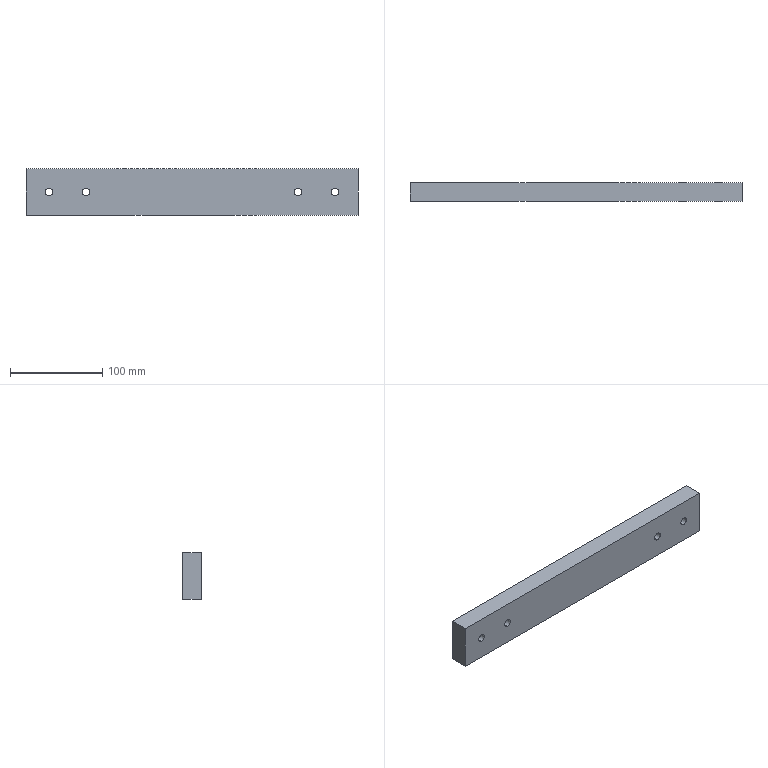Part | SolidWorks | features Extrusion 1, HoleWzd 1 | 1 solid | 14 faces | box 360 x 20 x 50 mm | volume 355460 mm3 | cylinder 8 | plane 6 | commonest cylinder face diameters 8.5 x8
STEP:
#1=CARTESIAN_POINT('',(335.,67.,-20.75));
#2=VERTEX_POINT('',#1);
#3=CARTESIAN_POINT('',(335.,67.,-29.25));
#4=VERTEX_POINT('',#3);
#5=CARTESIAN_POINT('',(335.,67.,-25.));
#6=DIRECTION('',(0.,-1.,0.));
#7=DIRECTION('',(0.,0.,-1.));
#8=AXIS2_PLACEMENT_3D('',#5,#6,#7);
#9=CIRCLE('',#8,4.25);
#10=EDGE_CURVE('',#2,#4,#9,.T.);
#11=ORIENTED_EDGE('',*,*,#10,.F.);
#12=CARTESIAN_POINT('',(335.,47.,-20.75));
#13=VERTEX_POINT('',#12);
#14=CARTESIAN_POINT('',(335.,47.,-20.75));
#15=DIRECTION('',(0.,-1.,0.));
#16=VECTOR('',#15,1000.);
#17=LINE('',#14,#16);
#18=EDGE_CURVE('',#2,#13,#17,.T.);
#19=ORIENTED_EDGE('',*,*,#18,.T.);
#20=CARTESIAN_POINT('',(335.,47.,-29.25));
#21=VERTEX_POINT('',#20);
#22=CARTESIAN_POINT('',(335.,47.,-25.));
#23=DIRECTION('',(0.,-1.,0.));
#24=DIRECTION('',(0.,0.,-1.));
#25=AXIS2_PLACEMENT_3D('',#22,#23,#24);
#26=CIRCLE('',#25,4.25);
#27=EDGE_CURVE('',#13,#21,#26,.T.);
#28=ORIENTED_EDGE('',*,*,#27,.T.);
#29=CARTESIAN_POINT('',(335.,47.,-29.25));
#30=DIRECTION('',(0.,-1.,0.));
#31=VECTOR('',#30,1000.);
#32=LINE('',#29,#31);
#33=EDGE_CURVE('',#4,#21,#32,.T.);
#34=ORIENTED_EDGE('',*,*,#33,.F.);
#35=EDGE_LOOP('',(#11,#19,#28,#34));
#36=FACE_OUTER_BOUND('',#35,.T.);
#37=CARTESIAN_POINT('',(335.,47.,-25.));
#38=DIRECTION('',(0.,-1.,0.));
#39=DIRECTION('',(0.,0.,-1.));
#40=AXIS2_PLACEMENT_3D('',#37,#38,#39);
#41=CYLINDRICAL_SURFACE('',#40,4.25);
#42=ADVANCED_FACE('',(#36),#41,.F.);
#43=CARTESIAN_POINT('',(295.,67.,-20.75));
#44=VERTEX_POINT('',#43);
#45=CARTESIAN_POINT('',(295.,67.,-29.25));
#46=VERTEX_POINT('',#45);
#47=CARTESIAN_POINT('',(295.,67.,-25.));
#48=DIRECTION('',(0.,-1.,0.));
#49=DIRECTION('',(0.,0.,-1.));
#50=AXIS2_PLACEMENT_3D('',#47,#48,#49);
#51=CIRCLE('',#50,4.25);
#52=EDGE_CURVE('',#44,#46,#51,.T.);
#53=ORIENTED_EDGE('',*,*,#52,.F.);
#54=CARTESIAN_POINT('',(295.,47.,-20.75));
#55=VERTEX_POINT('',#54);
#56=CARTESIAN_POINT('',(295.,47.,-20.75));
#57=DIRECTION('',(0.,-1.,0.));
#58=VECTOR('',#57,1000.);
#59=LINE('',#56,#58);
#60=EDGE_CURVE('',#44,#55,#59,.T.);
#61=ORIENTED_EDGE('',*,*,#60,.T.);
#62=CARTESIAN_POINT('',(295.,47.,-29.25));
#63=VERTEX_POINT('',#62);
#64=CARTESIAN_POINT('',(295.,47.,-25.));
#65=DIRECTION('',(0.,-1.,0.));
#66=DIRECTION('',(0.,0.,-1.));
#67=AXIS2_PLACEMENT_3D('',#64,#65,#66);
#68=CIRCLE('',#67,4.25);
#69=EDGE_CURVE('',#55,#63,#68,.T.);
#70=ORIENTED_EDGE('',*,*,#69,.T.);
#71=CARTESIAN_POINT('',(295.,47.,-29.25));
#72=DIRECTION('',(0.,-1.,0.));
#73=VECTOR('',#72,1000.);
#74=LINE('',#71,#73);
#75=EDGE_CURVE('',#46,#63,#74,.T.);
#76=ORIENTED_EDGE('',*,*,#75,.F.);
#77=EDGE_LOOP('',(#53,#61,#70,#76));
#78=FACE_OUTER_BOUND('',#77,.T.);
#79=CARTESIAN_POINT('',(295.,47.,-25.));
#80=DIRECTION('',(0.,-1.,0.));
#81=DIRECTION('',(0.,0.,-1.));
#82=AXIS2_PLACEMENT_3D('',#79,#80,#81);
#83=CYLINDRICAL_SURFACE('',#82,4.25);
#84=ADVANCED_FACE('',(#78),#83,.F.);
#85=CARTESIAN_POINT('',(65.,67.,-20.75));
#86=VERTEX_POINT('',#85);
#87=CARTESIAN_POINT('',(65.,67.,-29.25));
#88=VERTEX_POINT('',#87);
#89=CARTESIAN_POINT('',(65.,67.,-25.));
#90=DIRECTION('',(0.,-1.,0.));
#91=DIRECTION('',(0.,0.,-1.));
#92=AXIS2_PLACEMENT_3D('',#89,#90,#91);
#93=CIRCLE('',#92,4.25);
#94=EDGE_CURVE('',#86,#88,#93,.T.);
#95=ORIENTED_EDGE('',*,*,#94,.F.);
#96=CARTESIAN_POINT('',(65.,47.,-20.75));
#97=VERTEX_POINT('',#96);
#98=CARTESIAN_POINT('',(65.,47.,-20.75));
#99=DIRECTION('',(0.,-1.,0.));
#100=VECTOR('',#99,1000.);
#101=LINE('',#98,#100);
#102=EDGE_CURVE('',#86,#97,#101,.T.);
#103=ORIENTED_EDGE('',*,*,#102,.T.);
#104=CARTESIAN_POINT('',(65.,47.,-29.25));
#105=VERTEX_POINT('',#104);
#106=CARTESIAN_POINT('',(65.,47.,-25.));
#107=DIRECTION('',(0.,-1.,0.));
#108=DIRECTION('',(0.,0.,-1.));
#109=AXIS2_PLACEMENT_3D('',#106,#107,#108);
#110=CIRCLE('',#109,4.25);
#111=EDGE_CURVE('',#97,#105,#110,.T.);
#112=ORIENTED_EDGE('',*,*,#111,.T.);
#113=CARTESIAN_POINT('',(65.,47.,-29.25));
#114=DIRECTION('',(0.,-1.,0.));
#115=VECTOR('',#114,1000.);
#116=LINE('',#113,#115);
#117=EDGE_CURVE('',#88,#105,#116,.T.);
#118=ORIENTED_EDGE('',*,*,#117,.F.);
#119=EDGE_LOOP('',(#95,#103,#112,#118));
#120=FACE_OUTER_BOUND('',#119,.T.);
#121=CARTESIAN_POINT('',(65.,47.,-25.));
#122=DIRECTION('',(0.,-1.,0.));
#123=DIRECTION('',(0.,0.,-1.));
#124=AXIS2_PLACEMENT_3D('',#121,#122,#123);
#125=CYLINDRICAL_SURFACE('',#124,4.25);
#126=ADVANCED_FACE('',(#120),#125,.F.);
#127=CARTESIAN_POINT('',(25.,67.,-20.75));
#128=VERTEX_POINT('',#127);
#129=CARTESIAN_POINT('',(25.,67.,-29.25));
#130=VERTEX_POINT('',#129);
#131=CARTESIAN_POINT('',(25.,67.,-25.));
#132=DIRECTION('',(0.,-1.,0.));
#133=DIRECTION('',(0.,0.,-1.));
#134=AXIS2_PLACEMENT_3D('',#131,#132,#133);
#135=CIRCLE('',#134,4.25);
#136=EDGE_CURVE('',#128,#130,#135,.T.);
#137=ORIENTED_EDGE('',*,*,#136,.F.);
#138=CARTESIAN_POINT('',(25.,47.,-20.75));
#139=VERTEX_POINT('',#138);
#140=CARTESIAN_POINT('',(25.,47.,-20.75));
#141=DIRECTION('',(0.,-1.,0.));
#142=VECTOR('',#141,1000.);
#143=LINE('',#140,#142);
#144=EDGE_CURVE('',#128,#139,#143,.T.);
#145=ORIENTED_EDGE('',*,*,#144,.T.);
#146=CARTESIAN_POINT('',(25.,47.,-29.25));
#147=VERTEX_POINT('',#146);
#148=CARTESIAN_POINT('',(25.,47.,-25.));
#149=DIRECTION('',(0.,-1.,0.));
#150=DIRECTION('',(0.,0.,-1.));
#151=AXIS2_PLACEMENT_3D('',#148,#149,#150);
#152=CIRCLE('',#151,4.25);
#153=EDGE_CURVE('',#139,#147,#152,.T.);
#154=ORIENTED_EDGE('',*,*,#153,.T.);
#155=CARTESIAN_POINT('',(25.,47.,-29.25));
#156=DIRECTION('',(0.,-1.,0.));
#157=VECTOR('',#156,1000.);
#158=LINE('',#155,#157);
#159=EDGE_CURVE('',#130,#147,#158,.T.);
#160=ORIENTED_EDGE('',*,*,#159,.F.);
#161=EDGE_LOOP('',(#137,#145,#154,#160));
#162=FACE_OUTER_BOUND('',#161,.T.);
#163=CARTESIAN_POINT('',(25.,47.,-25.));
#164=DIRECTION('',(0.,-1.,0.));
#165=DIRECTION('',(0.,0.,-1.));
#166=AXIS2_PLACEMENT_3D('',#163,#164,#165);
#167=CYLINDRICAL_SURFACE('',#166,4.25);
#168=ADVANCED_FACE('',(#162),#167,.F.);
#169=CARTESIAN_POINT('',(360.,47.,-50.));
#170=VERTEX_POINT('',#169);
#171=CARTESIAN_POINT('',(360.,47.,0.));
#172=VERTEX_POINT('',#171);
#173=CARTESIAN_POINT('',(360.,47.,-50.));
#174=DIRECTION('',(0.,0.,1.));
#175=VECTOR('',#174,1000.);
#176=LINE('',#173,#175);
#177=EDGE_CURVE('',#170,#172,#176,.T.);
#178=ORIENTED_EDGE('',*,*,#177,.F.);
#179=CARTESIAN_POINT('',(360.,67.,-50.));
#180=VERTEX_POINT('',#179);
#181=CARTESIAN_POINT('',(360.,67.,-50.));
#182=DIRECTION('',(0.,-1.,0.));
#183=VECTOR('',#182,1000.);
#184=LINE('',#181,#183);
#185=EDGE_CURVE('',#180,#170,#184,.T.);
#186=ORIENTED_EDGE('',*,*,#185,.F.);
#187=CARTESIAN_POINT('',(360.,67.,0.));
#188=VERTEX_POINT('',#187);
#189=CARTESIAN_POINT('',(360.,67.,-50.));
#190=DIRECTION('',(0.,0.,1.));
#191=VECTOR('',#190,1000.);
#192=LINE('',#189,#191);
#193=EDGE_CURVE('',#180,#188,#192,.T.);
#194=ORIENTED_EDGE('',*,*,#193,.T.);
#195=CARTESIAN_POINT('',(360.,67.,0.));
#196=DIRECTION('',(0.,-1.,0.));
#197=VECTOR('',#196,1000.);
#198=LINE('',#195,#197);
#199=EDGE_CURVE('',#188,#172,#198,.T.);
#200=ORIENTED_EDGE('',*,*,#199,.T.);
#201=EDGE_LOOP('',(#178,#186,#194,#200));
#202=FACE_OUTER_BOUND('',#201,.T.);
#203=CARTESIAN_POINT('',(360.,67.,-50.));
#204=DIRECTION('',(1.,0.,0.));
#205=DIRECTION('',(0.,0.,-1.));
#206=AXIS2_PLACEMENT_3D('',#203,#204,#205);
#207=PLANE('',#206);
#208=ADVANCED_FACE('',(#202),#207,.T.);
#209=CARTESIAN_POINT('',(0.,47.,-50.));
#210=VERTEX_POINT('',#209);
#211=CARTESIAN_POINT('',(0.,47.,-50.));
#212=DIRECTION('',(1.,0.,0.));
#213=VECTOR('',#212,1000.);
#214=LINE('',#211,#213);
#215=EDGE_CURVE('',#210,#170,#214,.T.);
#216=ORIENTED_EDGE('',*,*,#215,.F.);
#217=CARTESIAN_POINT('',(0.,67.,-50.));
#218=VERTEX_POINT('',#217);
#219=CARTESIAN_POINT('',(0.,67.,-50.));
#220=DIRECTION('',(0.,-1.,0.));
#221=VECTOR('',#220,1000.);
#222=LINE('',#219,#221);
#223=EDGE_CURVE('',#218,#210,#222,.T.);
#224=ORIENTED_EDGE('',*,*,#223,.F.);
#225=CARTESIAN_POINT('',(0.,67.,-50.));
#226=DIRECTION('',(1.,0.,0.));
#227=VECTOR('',#226,1000.);
#228=LINE('',#225,#227);
#229=EDGE_CURVE('',#218,#180,#228,.T.);
#230=ORIENTED_EDGE('',*,*,#229,.T.);
#231=ORIENTED_EDGE('',*,*,#185,.T.);
#232=EDGE_LOOP('',(#216,#224,#230,#231));
#233=FACE_OUTER_BOUND('',#232,.T.);
#234=CARTESIAN_POINT('',(0.,67.,-50.));
#235=DIRECTION('',(0.,0.,-1.));
#236=DIRECTION('',(-1.,0.,0.));
#237=AXIS2_PLACEMENT_3D('',#234,#235,#236);
#238=PLANE('',#237);
#239=ADVANCED_FACE('',(#233),#238,.T.);
#240=CARTESIAN_POINT('',(0.,47.,0.));
#241=VERTEX_POINT('',#240);
#242=CARTESIAN_POINT('',(0.,47.,0.));
#243=DIRECTION('',(0.,0.,-1.));
#244=VECTOR('',#243,1000.);
#245=LINE('',#242,#244);
#246=EDGE_CURVE('',#241,#210,#245,.T.);
#247=ORIENTED_EDGE('',*,*,#246,.F.);
#248=CARTESIAN_POINT('',(0.,67.,0.));
#249=VERTEX_POINT('',#248);
#250=CARTESIAN_POINT('',(0.,67.,0.));
#251=DIRECTION('',(0.,-1.,0.));
#252=VECTOR('',#251,1000.);
#253=LINE('',#250,#252);
#254=EDGE_CURVE('',#249,#241,#253,.T.);
#255=ORIENTED_EDGE('',*,*,#254,.F.);
#256=CARTESIAN_POINT('',(0.,67.,0.));
#257=DIRECTION('',(0.,0.,-1.));
#258=VECTOR('',#257,1000.);
#259=LINE('',#256,#258);
#260=EDGE_CURVE('',#249,#218,#259,.T.);
#261=ORIENTED_EDGE('',*,*,#260,.T.);
#262=ORIENTED_EDGE('',*,*,#223,.T.);
#263=EDGE_LOOP('',(#247,#255,#261,#262));
#264=FACE_OUTER_BOUND('',#263,.T.);
#265=CARTESIAN_POINT('',(0.,67.,0.));
#266=DIRECTION('',(-1.,0.,0.));
#267=DIRECTION('',(0.,0.,1.));
#268=AXIS2_PLACEMENT_3D('',#265,#266,#267);
#269=PLANE('',#268);
#270=ADVANCED_FACE('',(#264),#269,.T.);
#271=CARTESIAN_POINT('',(360.,47.,0.));
#272=DIRECTION('',(-1.,0.,0.));
#273=VECTOR('',#272,1000.);
#274=LINE('',#271,#273);
#275=EDGE_CURVE('',#172,#241,#274,.T.);
#276=ORIENTED_EDGE('',*,*,#275,.F.);
#277=ORIENTED_EDGE('',*,*,#199,.F.);
#278=CARTESIAN_POINT('',(360.,67.,0.));
#279=DIRECTION('',(-1.,0.,0.));
#280=VECTOR('',#279,1000.);
#281=LINE('',#278,#280);
#282=EDGE_CURVE('',#188,#249,#281,.T.);
#283=ORIENTED_EDGE('',*,*,#282,.T.);
#284=ORIENTED_EDGE('',*,*,#254,.T.);
#285=EDGE_LOOP('',(#276,#277,#283,#284));
#286=FACE_OUTER_BOUND('',#285,.T.);
#287=CARTESIAN_POINT('',(360.,67.,0.));
#288=DIRECTION('',(0.,0.,1.));
#289=DIRECTION('',(1.,0.,0.));
#290=AXIS2_PLACEMENT_3D('',#287,#288,#289);
#291=PLANE('',#290);
#292=ADVANCED_FACE('',(#286),#291,.T.);
#293=CARTESIAN_POINT('',(335.,67.,-25.));
#294=DIRECTION('',(0.,-1.,0.));
#295=DIRECTION('',(0.,0.,-1.));
#296=AXIS2_PLACEMENT_3D('',#293,#294,#295);
#297=CIRCLE('',#296,4.25);
#298=EDGE_CURVE('',#4,#2,#297,.T.);
#299=ORIENTED_EDGE('',*,*,#298,.T.);
#300=ORIENTED_EDGE('',*,*,#10,.T.);
#301=EDGE_LOOP('',(#299,#300));
#302=FACE_BOUND('',#301,.T.);
#303=CARTESIAN_POINT('',(295.,67.,-25.));
#304=DIRECTION('',(0.,-1.,0.));
#305=DIRECTION('',(0.,0.,-1.));
#306=AXIS2_PLACEMENT_3D('',#303,#304,#305);
#307=CIRCLE('',#306,4.25);
#308=EDGE_CURVE('',#46,#44,#307,.T.);
#309=ORIENTED_EDGE('',*,*,#308,.T.);
#310=ORIENTED_EDGE('',*,*,#52,.T.);
#311=EDGE_LOOP('',(#309,#310));
#312=FACE_BOUND('',#311,.T.);
#313=CARTESIAN_POINT('',(65.,67.,-25.));
#314=DIRECTION('',(0.,-1.,0.));
#315=DIRECTION('',(0.,0.,-1.));
#316=AXIS2_PLACEMENT_3D('',#313,#314,#315);
#317=CIRCLE('',#316,4.25);
#318=EDGE_CURVE('',#88,#86,#317,.T.);
#319=ORIENTED_EDGE('',*,*,#318,.T.);
#320=ORIENTED_EDGE('',*,*,#94,.T.);
#321=EDGE_LOOP('',(#319,#320));
#322=FACE_BOUND('',#321,.T.);
#323=CARTESIAN_POINT('',(25.,67.,-25.));
#324=DIRECTION('',(0.,-1.,0.));
#325=DIRECTION('',(0.,0.,-1.));
#326=AXIS2_PLACEMENT_3D('',#323,#324,#325);
#327=CIRCLE('',#326,4.25);
#328=EDGE_CURVE('',#130,#128,#327,.T.);
#329=ORIENTED_EDGE('',*,*,#328,.T.);
#330=ORIENTED_EDGE('',*,*,#136,.T.);
#331=EDGE_LOOP('',(#329,#330));
#332=FACE_BOUND('',#331,.T.);
#333=ORIENTED_EDGE('',*,*,#193,.F.);
#334=ORIENTED_EDGE('',*,*,#229,.F.);
#335=ORIENTED_EDGE('',*,*,#260,.F.);
#336=ORIENTED_EDGE('',*,*,#282,.F.);
#337=EDGE_LOOP('',(#333,#334,#335,#336));
#338=FACE_OUTER_BOUND('',#337,.T.);
#339=CARTESIAN_POINT('',(0.,67.,0.));
#340=DIRECTION('',(0.,-1.,0.));
#341=DIRECTION('',(0.,0.,-1.));
#342=AXIS2_PLACEMENT_3D('',#339,#340,#341);
#343=PLANE('',#342);
#344=ADVANCED_FACE('',(#302,#312,#322,#332,#338),#343,.F.);
#345=CARTESIAN_POINT('',(335.,47.,-25.));
#346=DIRECTION('',(0.,-1.,0.));
#347=DIRECTION('',(0.,0.,-1.));
#348=AXIS2_PLACEMENT_3D('',#345,#346,#347);
#349=CIRCLE('',#348,4.25);
#350=EDGE_CURVE('',#21,#13,#349,.T.);
#351=ORIENTED_EDGE('',*,*,#350,.F.);
#352=ORIENTED_EDGE('',*,*,#27,.F.);
#353=EDGE_LOOP('',(#351,#352));
#354=FACE_BOUND('',#353,.T.);
#355=CARTESIAN_POINT('',(295.,47.,-25.));
#356=DIRECTION('',(0.,-1.,0.));
#357=DIRECTION('',(0.,0.,-1.));
#358=AXIS2_PLACEMENT_3D('',#355,#356,#357);
#359=CIRCLE('',#358,4.25);
#360=EDGE_CURVE('',#63,#55,#359,.T.);
#361=ORIENTED_EDGE('',*,*,#360,.F.);
#362=ORIENTED_EDGE('',*,*,#69,.F.);
#363=EDGE_LOOP('',(#361,#362));
#364=FACE_BOUND('',#363,.T.);
#365=CARTESIAN_POINT('',(65.,47.,-25.));
#366=DIRECTION('',(0.,-1.,0.));
#367=DIRECTION('',(0.,0.,-1.));
#368=AXIS2_PLACEMENT_3D('',#365,#366,#367);
#369=CIRCLE('',#368,4.25);
#370=EDGE_CURVE('',#105,#97,#369,.T.);
#371=ORIENTED_EDGE('',*,*,#370,.F.);
#372=ORIENTED_EDGE('',*,*,#111,.F.);
#373=EDGE_LOOP('',(#371,#372));
#374=FACE_BOUND('',#373,.T.);
#375=CARTESIAN_POINT('',(25.,47.,-25.));
#376=DIRECTION('',(0.,-1.,0.));
#377=DIRECTION('',(0.,0.,-1.));
#378=AXIS2_PLACEMENT_3D('',#375,#376,#377);
#379=CIRCLE('',#378,4.25);
#380=EDGE_CURVE('',#147,#139,#379,.T.);
#381=ORIENTED_EDGE('',*,*,#380,.F.);
#382=ORIENTED_EDGE('',*,*,#153,.F.);
#383=EDGE_LOOP('',(#381,#382));
#384=FACE_BOUND('',#383,.T.);
#385=ORIENTED_EDGE('',*,*,#177,.T.);
#386=ORIENTED_EDGE('',*,*,#275,.T.);
#387=ORIENTED_EDGE('',*,*,#246,.T.);
#388=ORIENTED_EDGE('',*,*,#215,.T.);
#389=EDGE_LOOP('',(#385,#386,#387,#388));
#390=FACE_OUTER_BOUND('',#389,.T.);
#391=CARTESIAN_POINT('',(0.,47.,0.));
#392=DIRECTION('',(0.,-1.,0.));
#393=DIRECTION('',(0.,0.,-1.));
#394=AXIS2_PLACEMENT_3D('',#391,#392,#393);
#395=PLANE('',#394);
#396=ADVANCED_FACE('',(#354,#364,#374,#384,#390),#395,.T.);
#397=ORIENTED_EDGE('',*,*,#144,.F.);
#398=ORIENTED_EDGE('',*,*,#328,.F.);
#399=ORIENTED_EDGE('',*,*,#159,.T.);
#400=ORIENTED_EDGE('',*,*,#380,.T.);
#401=EDGE_LOOP('',(#397,#398,#399,#400));
#402=FACE_OUTER_BOUND('',#401,.T.);
#403=CARTESIAN_POINT('',(25.,47.,-25.));
#404=DIRECTION('',(0.,-1.,0.));
#405=DIRECTION('',(0.,0.,-1.));
#406=AXIS2_PLACEMENT_3D('',#403,#404,#405);
#407=CYLINDRICAL_SURFACE('',#406,4.25);
#408=ADVANCED_FACE('',(#402),#407,.F.);
#409=ORIENTED_EDGE('',*,*,#102,.F.);
#410=ORIENTED_EDGE('',*,*,#318,.F.);
#411=ORIENTED_EDGE('',*,*,#117,.T.);
#412=ORIENTED_EDGE('',*,*,#370,.T.);
#413=EDGE_LOOP('',(#409,#410,#411,#412));
#414=FACE_OUTER_BOUND('',#413,.T.);
#415=CARTESIAN_POINT('',(65.,47.,-25.));
#416=DIRECTION('',(0.,-1.,0.));
#417=DIRECTION('',(0.,0.,-1.));
#418=AXIS2_PLACEMENT_3D('',#415,#416,#417);
#419=CYLINDRICAL_SURFACE('',#418,4.25);
#420=ADVANCED_FACE('',(#414),#419,.F.);
#421=ORIENTED_EDGE('',*,*,#60,.F.);
#422=ORIENTED_EDGE('',*,*,#308,.F.);
#423=ORIENTED_EDGE('',*,*,#75,.T.);
#424=ORIENTED_EDGE('',*,*,#360,.T.);
#425=EDGE_LOOP('',(#421,#422,#423,#424));
#426=FACE_OUTER_BOUND('',#425,.T.);
#427=CARTESIAN_POINT('',(295.,47.,-25.));
#428=DIRECTION('',(0.,-1.,0.));
#429=DIRECTION('',(0.,0.,-1.));
#430=AXIS2_PLACEMENT_3D('',#427,#428,#429);
#431=CYLINDRICAL_SURFACE('',#430,4.25);
#432=ADVANCED_FACE('',(#426),#431,.F.);
#433=ORIENTED_EDGE('',*,*,#18,.F.);
#434=ORIENTED_EDGE('',*,*,#298,.F.);
#435=ORIENTED_EDGE('',*,*,#33,.T.);
#436=ORIENTED_EDGE('',*,*,#350,.T.);
#437=EDGE_LOOP('',(#433,#434,#435,#436));
#438=FACE_OUTER_BOUND('',#437,.T.);
#439=CARTESIAN_POINT('',(335.,47.,-25.));
#440=DIRECTION('',(0.,-1.,0.));
#441=DIRECTION('',(0.,0.,-1.));
#442=AXIS2_PLACEMENT_3D('',#439,#440,#441);
#443=CYLINDRICAL_SURFACE('',#442,4.25);
#444=ADVANCED_FACE('',(#438),#443,.F.);
#445=CLOSED_SHELL('',(#42,#84,#126,#168,#208,#239,#270,#292,#344,#396,#408,#420,#432,#444));
#446=MANIFOLD_SOLID_BREP('',#445);
#447=CARTESIAN_POINT('',(0.,0.,0.));
#448=DIRECTION('',(0.,0.,1.));
#449=DIRECTION('',(1.,0.,0.));
#450=AXIS2_PLACEMENT_3D('',#447,#448,#449);
#451=(LENGTH_UNIT()NAMED_UNIT(*)SI_UNIT(.MILLI.,.METRE.));
#452=UNCERTAINTY_MEASURE_WITH_UNIT(LENGTH_MEASURE(0.00001),#451,'','');
#453=(NAMED_UNIT(*)PLANE_ANGLE_UNIT()SI_UNIT($,.RADIAN.));
#454=(NAMED_UNIT(*)SI_UNIT($,.STERADIAN.)SOLID_ANGLE_UNIT());
#455=(GEOMETRIC_REPRESENTATION_CONTEXT(3)GLOBAL_UNCERTAINTY_ASSIGNED_CONTEXT((#452))GLOBAL_UNIT_ASSIGNED_CONTEXT((#451,#453,#454))REPRESENTATION_CONTEXT('',''));
#456=ADVANCED_BREP_SHAPE_REPRESENTATION('',(#446,#450),#455);